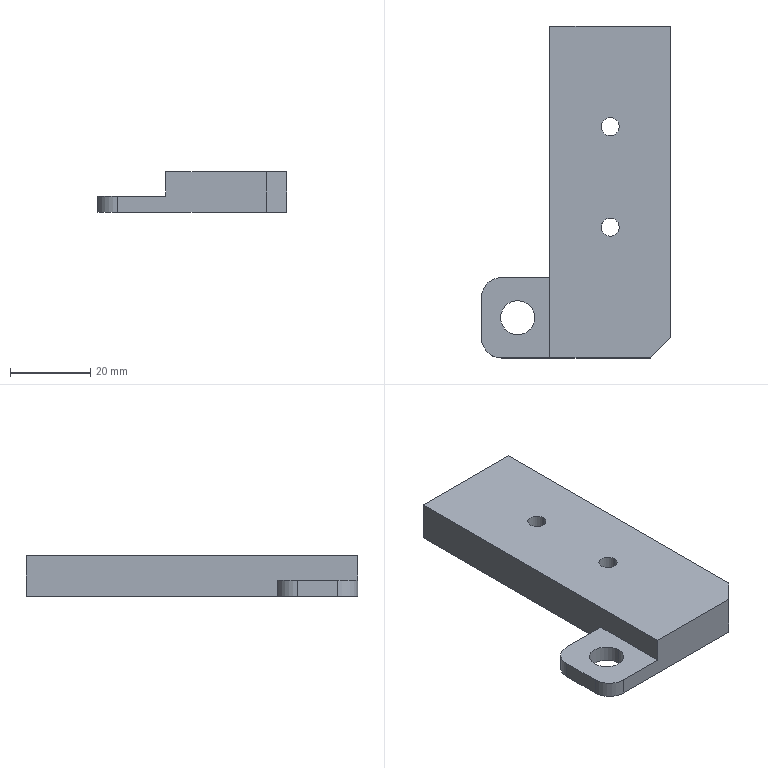Part | STEP file | 2071 Cylinder mounting plate 13 | 1 solid | 32 faces | box 47 x 82.5 x 10 mm | volume 24879 mm3 | cylinder 16 | plane 12 | cone 4 | commonest cylinder face diameters 3.3 x4 4.5 x4 8 x4 8.5 x2 10 x2